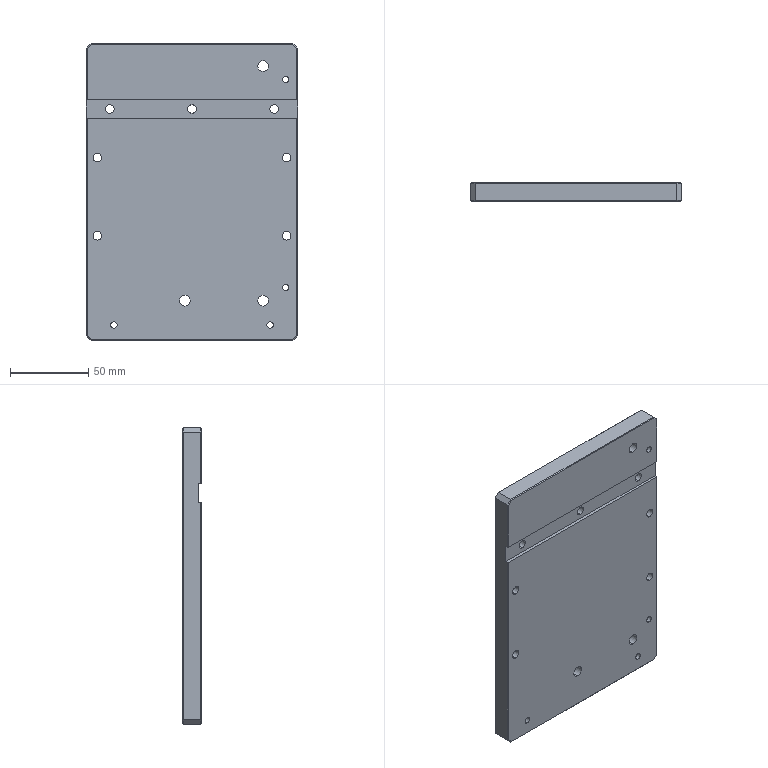Part | STEP file | ND25021-01-JDKM-42-TL | 1 solid | 87 faces | box 135 x 12 x 190 mm | volume 298236 mm3 | cylinder 46 | plane 41 | commonest cylinder face diameters 5.5 x14 10 x14 6.8 x6 4 x4 4.2 x4 5 x4